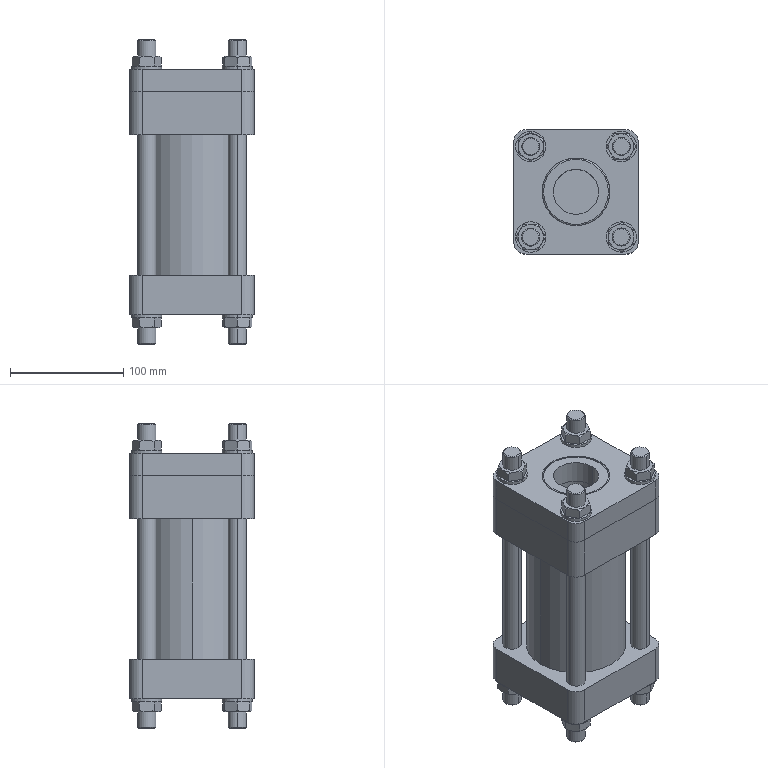Part | SolidWorks | features BaseBody 6 | 6 solids | 267 faces | box 110 x 110 x 269.096 mm | volume 1870008 mm3 | plane 103 | cylinder 90 | cone 72 | torus 2 | commonest cylinder face diameters 16 x48 26.88 x16 22 x12 19.793 x4 40 x4 59.8 x2